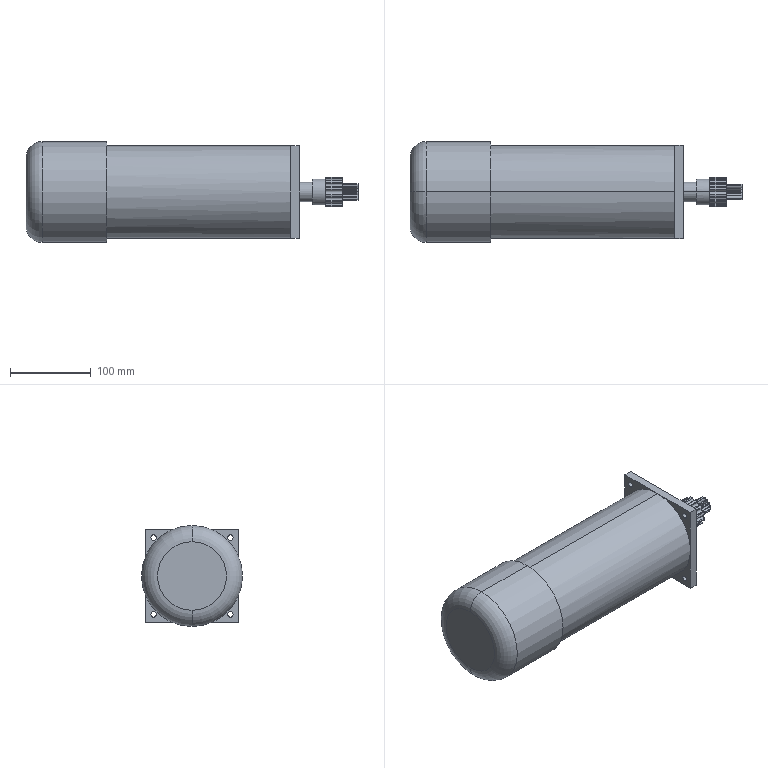Part | SolidWorks | features ICE 8, CirPattern 2, 3DProfileFeature 1, Extrusion 1, Fillet 1, HoleWzd 1, RefAxis 1 | 1 solid | 172 faces | box 411 x 125 x 125 mm | volume 3738771 mm3 | cylinder 104 | plane 38 | spline 28 | torus 2 | commonest cylinder face diameters 1.6 x30 5.14 x17 20 x15 14.375 x14 37 x12 6.8 x8